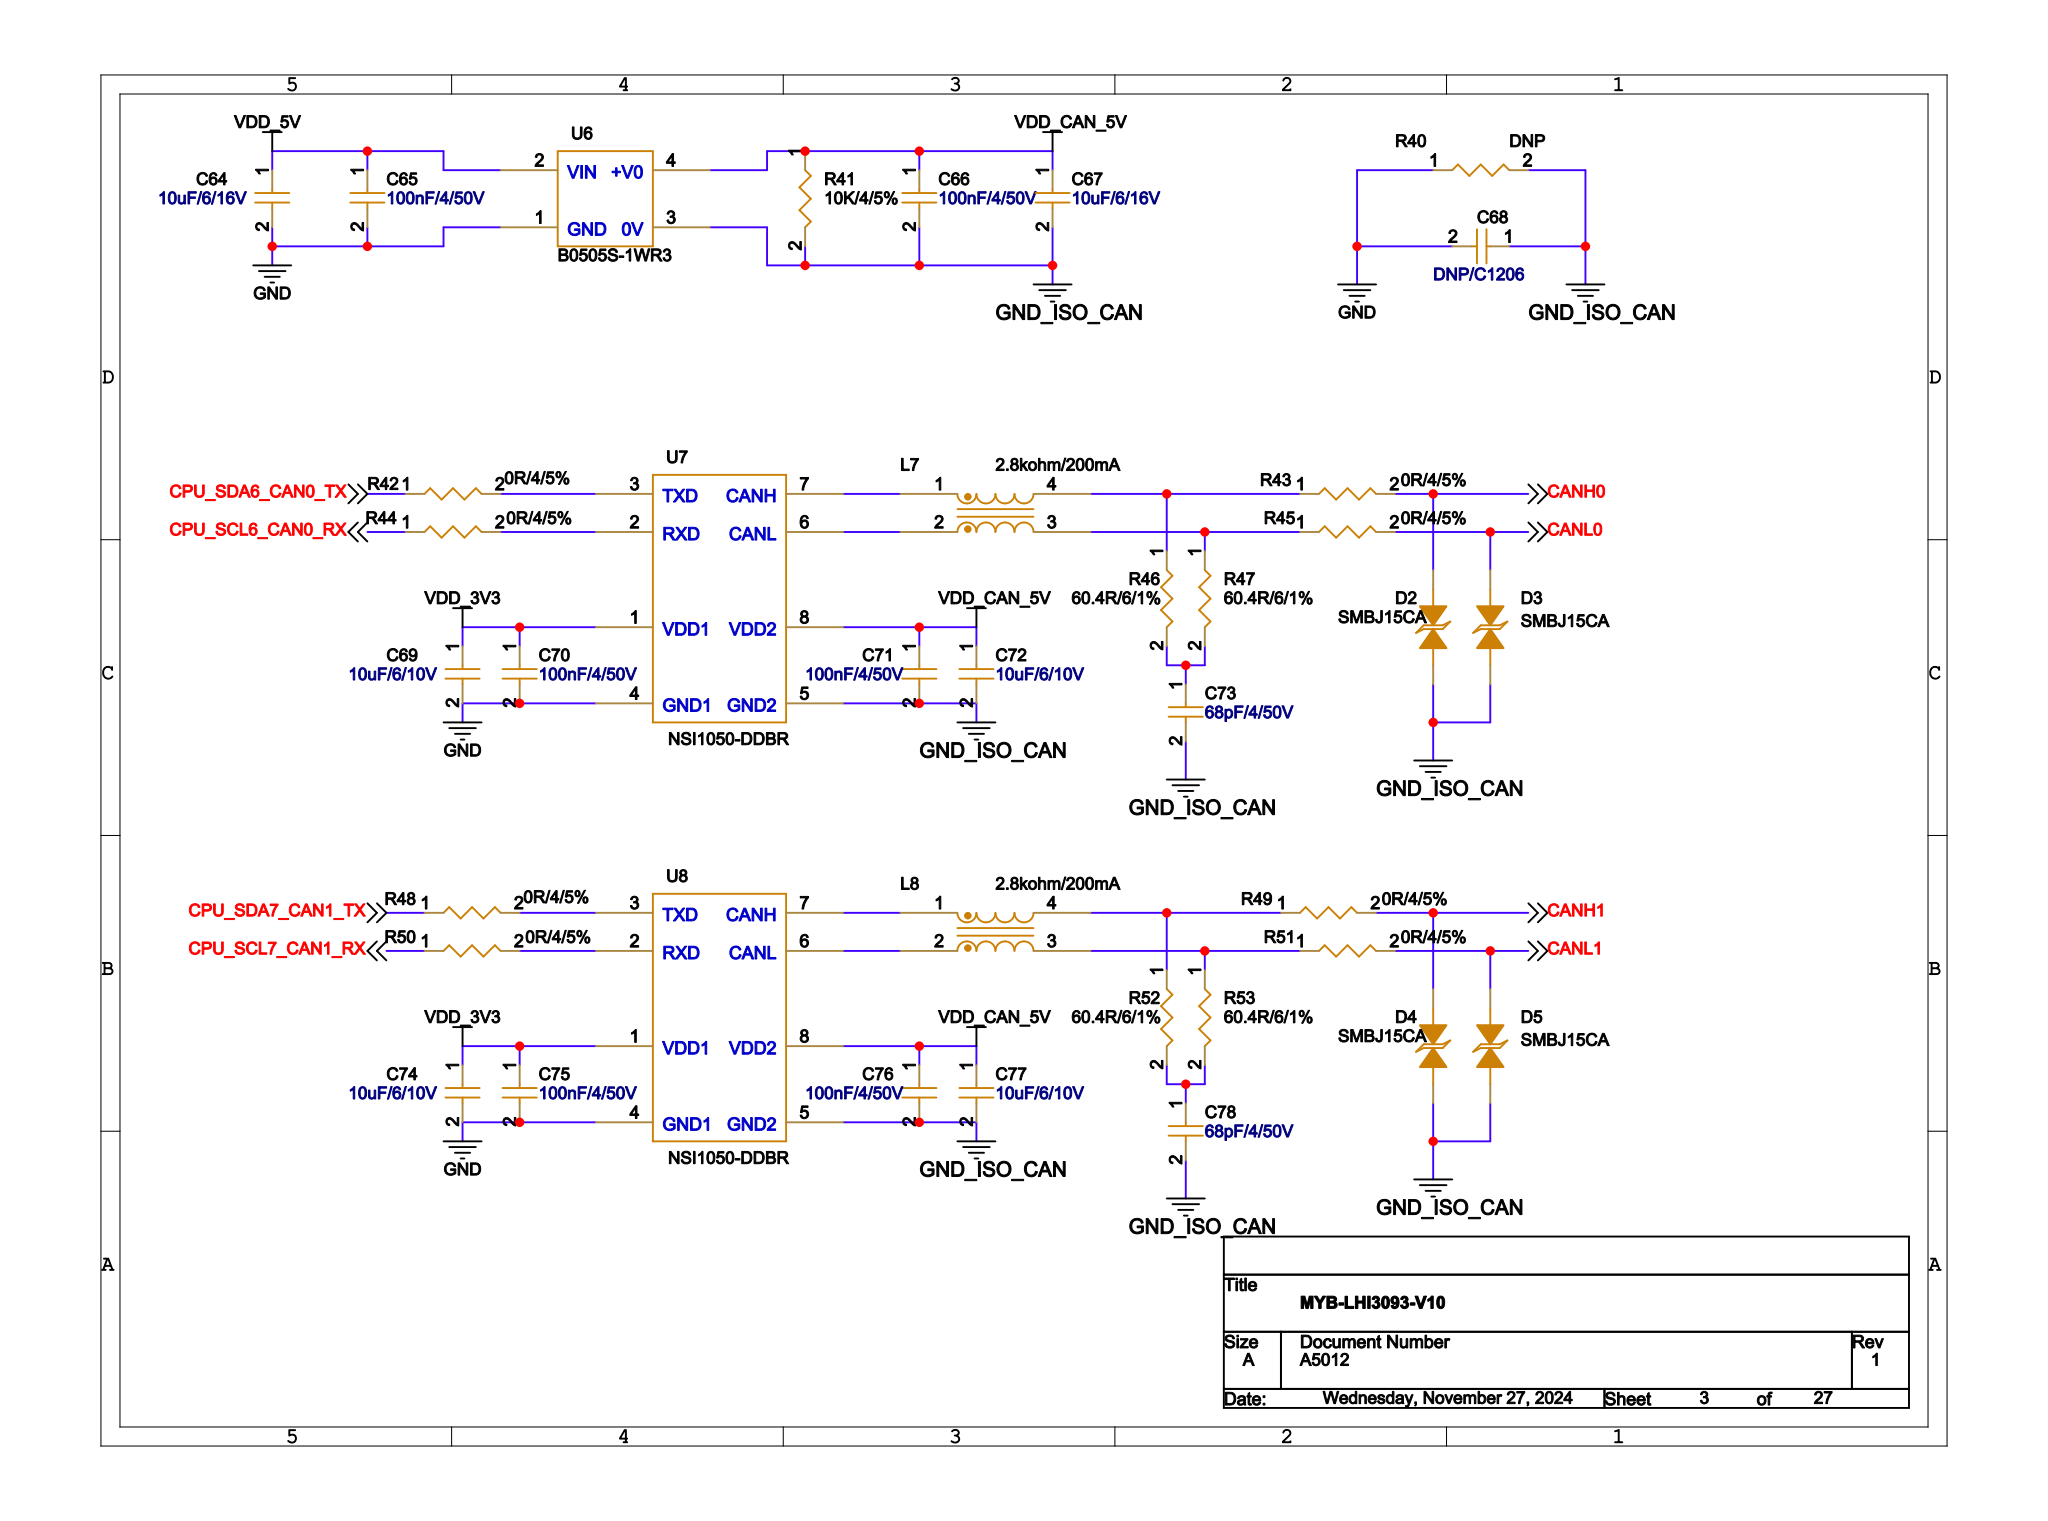Circuit board | Cadence Allegro | 1159 parts | 708 nets | one sheet of the schematic
Parts on this sheet (reference | value | footprint):
C64 | 10uF/6/16V | C0603
C65 | 100nF/4/50V | C0402
C66 | 100nF/4/50V | C0402
C67 | 10uF/6/16V | C0603
C68 | DNP/C1206 | C1206
C69 | 10uF/6/10V | C0603
C70 | 100nF/4/50V | C0402
C71 | 100nF/4/50V | C0402
C72 | 10uF/6/10V | C0603
C73 | 68pF/4/50V | C0402
C74 | 10uF/6/10V | C0603
C75 | 100nF/4/50V | C0402
C76 | 100nF/4/50V | C0402
C77 | 10uF/6/10V | C0603
C78 | 68pF/4/50V | C0402
D2 | SMBJ15CA | DO-214AA
D3 | SMBJ15CA | DO-214AA
D4 | SMBJ15CA | DO-214AA
D5 | SMBJ15CA | DO-214AA
L7 | 2.8kohm/200mA | INDCM-ACT45B
L8 | 2.8kohm/200mA | INDCM-ACT45B
R40 | DNP | R1206
R41 | 10K/4/5% | R0402
R42 | 0R/4/5% | R0402
R43 | 0R/4/5% | R0402
R44 | 0R/4/5% | R0402
R46 | 60.4R/6/1% | R0603
R47 | 60.4R/6/1% | R0603
R48 | 0R/4/5% | R0402
R49 | 0R/4/5% | R0402
R50 | 0R/4/5% | R0402
R52 | 60.4R/6/1% | R0603
R53 | 60.4R/6/1% | R0603
R451 | 1K/4/5% | R0402
R511 | 2K/4/1% | R0402
U6 | B0505S-1WR3 | MODULE-B0505S
U7 | NSI1050-DDBR | SOP8-2_54
U8 | NSI1050-DDBR | SOP8-2_54
Nets of these parts (net: part-pin ...):
GND: C64-2 C65-2 C68-2 C69-2 C70-2 C74-2 C75-2 R40-1 R451-1 U6-1 U7-4 U8-4
VDD_5V: C64-1 C65-1 U6-2
VDD_3V3: C69-1 C70-1 C74-1 C75-1 U7-1 U8-1
VDD_CAN_5V: C66-1 C67-1 C71-1 C72-1 C76-1 C77-1 R41-1 U6-4 U7-8 U8-8
GND_ISO_CAN: C66-2 C67-2 C68-1 C71-2 C72-2 C73-2 C76-2 C77-2 C78-2 D2-1 D3-1 D4-1 D5-1 R40-2 R41-2 U6-3 U7-5 U8-5
CPU_ADC_VIN14: R511-2
N14860085: C73-1 R46-2 R47-2
N14860980: C78-1 R52-2 R53-2
CANH0: D2-2 R43-2
CANL0: D3-2
CANH1: D4-2 R49-2
CANL1: D5-2
CPU_ADC_14_CON: R511-1
N14859851: L7-1 U7-7
N14859855: L7-2 U7-6
N14859923: L7-3 R47-1
N14859919: L7-4 R43-1 R46-1
N14860842: L8-1 U8-7
N14860846: L8-2 U8-6
N14860914: L8-3 R53-1
N14860890: L8-4 R49-1 R52-1
CPU_SDA6_CAN0_TX: R42-1
N14859610: R42-2 U7-3
CPU_SCL6_CAN0_RX: R44-1
N14859614: R44-2 U7-2
CPU_SDA7_CAN1_TX: R48-1
N14861348: R48-2 U8-3
CPU_SCL7_CAN1_RX: R50-1
N14861352: R50-2 U8-2
N15061726: R451-2